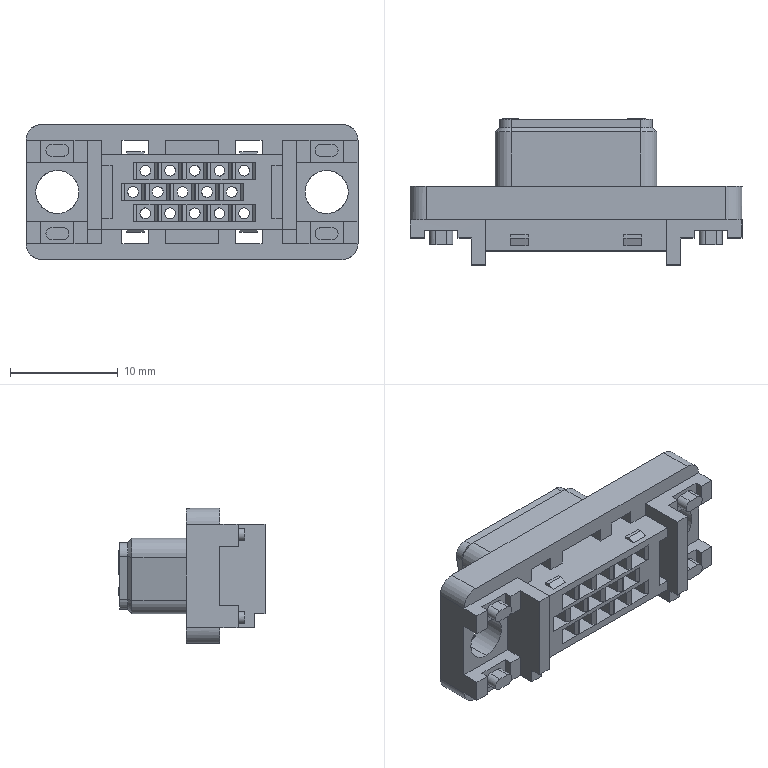Part | STEP file | HOUSING | 1 solid | 582 faces | box 30.8 x 13.55 x 12.55 mm | volume 1641 mm3 | plane 490 | cylinder 58 | cone 34 | commonest cylinder face diameters 1 x30 1.12 x8 3 x8 2.2 x4 4 x4 5.2 x4